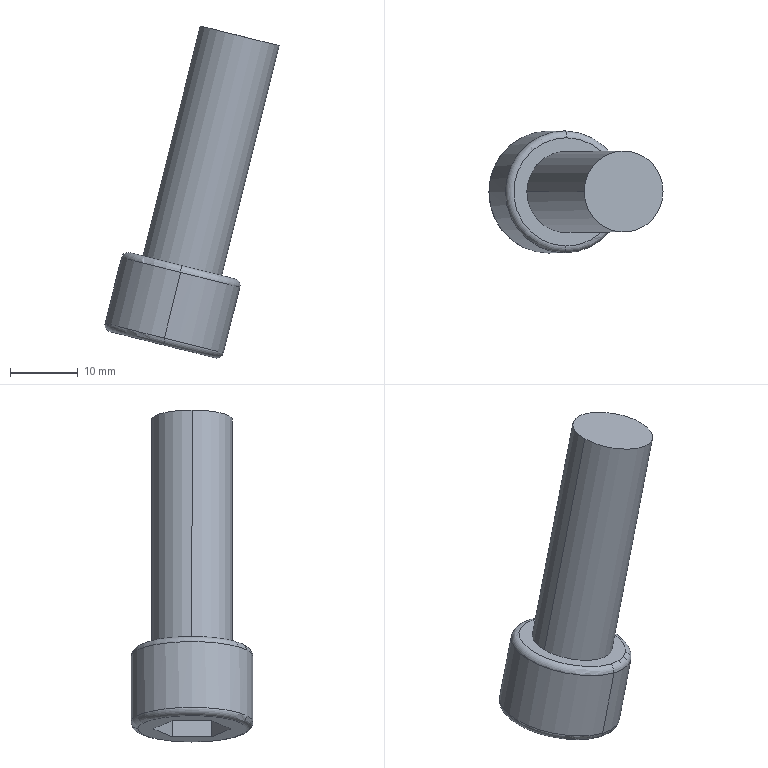Part | SolidWorks | features BaseBody 1 | 1 solid | 18 faces | box 25.711 x 18 x 49.02 mm | volume 6296 mm3 | plane 10 | torus 4 | cylinder 4 | commonest cylinder face diameters 12 x2 18 x2
STEP:
#1=CARTESIAN_POINT('',(-480.925,5.,189.664));
#2=VERTEX_POINT('',#1);
#3=CARTESIAN_POINT('',(-481.005,-13.,189.684));
#4=VERTEX_POINT('',#3);
#5=CARTESIAN_POINT('',(-480.925,-4.,189.664));
#6=DIRECTION('',(0.2419,0.,0.9703));
#7=DIRECTION('',(0.,-1.,0.));
#8=AXIS2_PLACEMENT_3D('',#5,#6,#7);
#9=CIRCLE('',#8,9.);
#10=EDGE_CURVE('',#2,#4,#9,.T.);
#11=ORIENTED_EDGE('',*,*,#10,.T.);
#12=CARTESIAN_POINT('',(-480.754,-12.,190.652));
#13=VERTEX_POINT('',#12);
#14=CARTESIAN_POINT('',(-480.996,-12.,189.681));
#15=DIRECTION('',(-0.9703,0.009133,0.2419));
#16=DIRECTION('',(0.2419,0.,0.9703));
#17=AXIS2_PLACEMENT_3D('',#14,#15,#16);
#18=CIRCLE('',#17,1.);
#19=EDGE_CURVE('',#4,#13,#18,.T.);
#20=ORIENTED_EDGE('',*,*,#19,.T.);
#21=CARTESIAN_POINT('',(-480.613,4.,190.616));
#22=VERTEX_POINT('',#21);
#23=CARTESIAN_POINT('',(-480.684,-4.,190.634));
#24=DIRECTION('',(0.2419,0.,0.9703));
#25=DIRECTION('',(0.,-1.,0.));
#26=AXIS2_PLACEMENT_3D('',#23,#24,#25);
#27=CIRCLE('',#26,8.);
#28=EDGE_CURVE('',#22,#13,#27,.T.);
#29=ORIENTED_EDGE('',*,*,#28,.F.);
#30=CARTESIAN_POINT('',(-480.846,5.,189.644));
#31=VERTEX_POINT('',#30);
#32=CARTESIAN_POINT('',(-480.855,4.,189.646));
#33=DIRECTION('',(0.9703,-0.009133,-0.2419));
#34=DIRECTION('',(-0.2419,0.,-0.9703));
#35=AXIS2_PLACEMENT_3D('',#32,#33,#34);
#36=CIRCLE('',#35,1.);
#37=EDGE_CURVE('',#31,#22,#36,.T.);
#38=ORIENTED_EDGE('',*,*,#37,.F.);
#39=CARTESIAN_POINT('',(-480.925,-4.,189.664));
#40=DIRECTION('',(0.2419,0.,0.9703));
#41=DIRECTION('',(0.,-1.,0.));
#42=AXIS2_PLACEMENT_3D('',#39,#40,#41);
#43=CIRCLE('',#42,9.);
#44=EDGE_CURVE('',#31,#2,#43,.T.);
#45=ORIENTED_EDGE('',*,*,#44,.T.);
#46=EDGE_LOOP('',(#11,#20,#29,#38,#45));
#47=FACE_OUTER_BOUND('',#46,.T.);
#48=CARTESIAN_POINT('',(-480.925,-4.,189.664));
#49=DIRECTION('',(0.2419,0.,0.9703));
#50=DIRECTION('',(0.008862,1.,-0.002209));
#51=AXIS2_PLACEMENT_3D('',#48,#49,#50);
#52=TOROIDAL_SURFACE('',#51,8.,1.);
#53=ADVANCED_FACE('',(#47),#52,.T.);
#54=CARTESIAN_POINT('',(-483.485,-11.999,178.965));
#55=VERTEX_POINT('',#54);
#56=CARTESIAN_POINT('',(-483.687,3.999,179.015));
#57=VERTEX_POINT('',#56);
#58=CARTESIAN_POINT('',(-483.586,-4.,178.99));
#59=DIRECTION('',(-0.2419,0.,-0.9703));
#60=DIRECTION('',(0.,-1.,0.));
#61=AXIS2_PLACEMENT_3D('',#58,#59,#60);
#62=CIRCLE('',#61,8.);
#63=EDGE_CURVE('',#55,#57,#62,.T.);
#64=ORIENTED_EDGE('',*,*,#63,.F.);
#65=CARTESIAN_POINT('',(-483.231,-12.999,179.932));
#66=VERTEX_POINT('',#65);
#67=CARTESIAN_POINT('',(-483.244,-11.999,179.936));
#68=DIRECTION('',(-0.9702,-0.01297,0.2419));
#69=DIRECTION('',(0.2419,0.,0.9703));
#70=AXIS2_PLACEMENT_3D('',#67,#68,#69);
#71=CIRCLE('',#70,1.);
#72=EDGE_CURVE('',#55,#66,#71,.T.);
#73=ORIENTED_EDGE('',*,*,#72,.T.);
#74=CARTESIAN_POINT('',(-483.344,-13.,179.961));
#75=VERTEX_POINT('',#74);
#76=CARTESIAN_POINT('',(-483.344,-4.,179.961));
#77=DIRECTION('',(-0.2419,0.,-0.9703));
#78=DIRECTION('',(0.,-1.,0.));
#79=AXIS2_PLACEMENT_3D('',#76,#77,#78);
#80=CIRCLE('',#79,9.);
#81=EDGE_CURVE('',#66,#75,#80,.T.);
#82=ORIENTED_EDGE('',*,*,#81,.T.);
#83=CARTESIAN_POINT('',(-483.458,4.999,179.989));
#84=VERTEX_POINT('',#83);
#85=CARTESIAN_POINT('',(-483.344,-4.,179.961));
#86=DIRECTION('',(-0.2419,0.,-0.9703));
#87=DIRECTION('',(0.,-1.,0.));
#88=AXIS2_PLACEMENT_3D('',#85,#86,#87);
#89=CIRCLE('',#88,9.);
#90=EDGE_CURVE('',#75,#84,#89,.T.);
#91=ORIENTED_EDGE('',*,*,#90,.T.);
#92=CARTESIAN_POINT('',(-483.445,3.999,179.986));
#93=DIRECTION('',(0.9702,0.01297,-0.2419));
#94=DIRECTION('',(-0.2419,0.,-0.9703));
#95=AXIS2_PLACEMENT_3D('',#92,#93,#94);
#96=CIRCLE('',#95,1.);
#97=EDGE_CURVE('',#57,#84,#96,.T.);
#98=ORIENTED_EDGE('',*,*,#97,.F.);
#99=EDGE_LOOP('',(#64,#73,#82,#91,#98));
#100=FACE_OUTER_BOUND('',#99,.T.);
#101=CARTESIAN_POINT('',(-483.344,-4.,179.961));
#102=DIRECTION('',(0.2419,0.,0.9703));
#103=DIRECTION('',(-0.01259,0.9999,0.003138));
#104=AXIS2_PLACEMENT_3D('',#101,#102,#103);
#105=TOROIDAL_SURFACE('',#104,8.,1.);
#106=ADVANCED_FACE('',(#100),#105,.T.);
#107=CARTESIAN_POINT('',(-483.344,5.,179.961));
#108=VERTEX_POINT('',#107);
#109=CARTESIAN_POINT('',(-483.344,-4.,179.961));
#110=DIRECTION('',(-0.2419,0.,-0.9703));
#111=DIRECTION('',(0.,-1.,0.));
#112=AXIS2_PLACEMENT_3D('',#109,#110,#111);
#113=CIRCLE('',#112,9.);
#114=EDGE_CURVE('',#108,#66,#113,.T.);
#115=ORIENTED_EDGE('',*,*,#114,.F.);
#116=CARTESIAN_POINT('',(-480.684,5.,190.634));
#117=DIRECTION('',(0.2419,0.,0.9703));
#118=VECTOR('',#117,1000.);
#119=LINE('',#116,#118);
#120=EDGE_CURVE('',#108,#2,#119,.T.);
#121=ORIENTED_EDGE('',*,*,#120,.T.);
#122=ORIENTED_EDGE('',*,*,#44,.F.);
#123=CARTESIAN_POINT('',(-480.925,-13.,189.664));
#124=VERTEX_POINT('',#123);
#125=CARTESIAN_POINT('',(-480.925,-4.,189.664));
#126=DIRECTION('',(0.2419,0.,0.9703));
#127=DIRECTION('',(0.,-1.,0.));
#128=AXIS2_PLACEMENT_3D('',#125,#126,#127);
#129=CIRCLE('',#128,9.);
#130=EDGE_CURVE('',#124,#31,#129,.T.);
#131=ORIENTED_EDGE('',*,*,#130,.F.);
#132=CARTESIAN_POINT('',(-480.684,-13.,190.634));
#133=DIRECTION('',(0.2419,0.,0.9703));
#134=VECTOR('',#133,1000.);
#135=LINE('',#132,#134);
#136=EDGE_CURVE('',#75,#124,#135,.T.);
#137=ORIENTED_EDGE('',*,*,#136,.F.);
#138=ORIENTED_EDGE('',*,*,#81,.F.);
#139=EDGE_LOOP('',(#115,#121,#122,#131,#137,#138));
#140=FACE_OUTER_BOUND('',#139,.T.);
#141=CARTESIAN_POINT('',(-480.684,-4.,190.634));
#142=DIRECTION('',(0.2419,0.,0.9703));
#143=DIRECTION('',(0.,-1.,0.));
#144=AXIS2_PLACEMENT_3D('',#141,#142,#143);
#145=CYLINDRICAL_SURFACE('',#144,9.);
#146=ADVANCED_FACE('',(#140),#145,.T.);
#147=CARTESIAN_POINT('',(-474.862,-4.,189.183));
#148=VERTEX_POINT('',#147);
#149=CARTESIAN_POINT('',(-486.505,-4.,192.085));
#150=VERTEX_POINT('',#149);
#151=CARTESIAN_POINT('',(-480.684,-4.,190.634));
#152=DIRECTION('',(0.2419,0.,0.9703));
#153=DIRECTION('',(0.9703,0.,-0.2419));
#154=AXIS2_PLACEMENT_3D('',#151,#152,#153);
#155=CIRCLE('',#154,6.);
#156=EDGE_CURVE('',#148,#150,#155,.T.);
#157=ORIENTED_EDGE('',*,*,#156,.T.);
#158=CARTESIAN_POINT('',(-478.039,-4.,226.046));
#159=VERTEX_POINT('',#158);
#160=CARTESIAN_POINT('',(-478.039,-4.,226.046));
#161=DIRECTION('',(0.2419,0.,0.9703));
#162=VECTOR('',#161,1000.);
#163=LINE('',#160,#162);
#164=EDGE_CURVE('',#150,#159,#163,.T.);
#165=ORIENTED_EDGE('',*,*,#164,.T.);
#166=CARTESIAN_POINT('',(-466.396,-4.,223.143));
#167=VERTEX_POINT('',#166);
#168=CARTESIAN_POINT('',(-472.218,-4.,224.595));
#169=DIRECTION('',(0.2419,0.,0.9703));
#170=DIRECTION('',(0.9703,0.,-0.2419));
#171=AXIS2_PLACEMENT_3D('',#168,#169,#170);
#172=CIRCLE('',#171,6.);
#173=EDGE_CURVE('',#167,#159,#172,.T.);
#174=ORIENTED_EDGE('',*,*,#173,.F.);
#175=CARTESIAN_POINT('',(-466.396,-4.,223.143));
#176=DIRECTION('',(0.2419,0.,0.9703));
#177=VECTOR('',#176,1000.);
#178=LINE('',#175,#177);
#179=EDGE_CURVE('',#148,#167,#178,.T.);
#180=ORIENTED_EDGE('',*,*,#179,.F.);
#181=EDGE_LOOP('',(#157,#165,#174,#180));
#182=FACE_OUTER_BOUND('',#181,.T.);
#183=CARTESIAN_POINT('',(-472.218,-4.,224.595));
#184=DIRECTION('',(0.2419,0.,0.9703));
#185=DIRECTION('',(0.9703,0.,-0.2419));
#186=AXIS2_PLACEMENT_3D('',#183,#184,#185);
#187=CYLINDRICAL_SURFACE('',#186,6.);
#188=ADVANCED_FACE('',(#182),#187,.T.);
#189=ORIENTED_EDGE('',*,*,#156,.F.);
#190=CARTESIAN_POINT('',(-480.684,-4.,190.634));
#191=DIRECTION('',(0.2419,0.,0.9703));
#192=DIRECTION('',(0.9703,0.,-0.2419));
#193=AXIS2_PLACEMENT_3D('',#190,#191,#192);
#194=CIRCLE('',#193,6.);
#195=EDGE_CURVE('',#150,#148,#194,.T.);
#196=ORIENTED_EDGE('',*,*,#195,.F.);
#197=EDGE_LOOP('',(#189,#196));
#198=FACE_BOUND('',#197,.T.);
#199=ORIENTED_EDGE('',*,*,#28,.T.);
#200=CARTESIAN_POINT('',(-480.684,-4.,190.634));
#201=DIRECTION('',(0.2419,0.,0.9703));
#202=DIRECTION('',(0.,-1.,0.));
#203=AXIS2_PLACEMENT_3D('',#200,#201,#202);
#204=CIRCLE('',#203,8.);
#205=EDGE_CURVE('',#13,#22,#204,.T.);
#206=ORIENTED_EDGE('',*,*,#205,.T.);
#207=EDGE_LOOP('',(#199,#206));
#208=FACE_OUTER_BOUND('',#207,.T.);
#209=CARTESIAN_POINT('',(-480.684,-4.,190.634));
#210=DIRECTION('',(0.2419,0.,0.9703));
#211=DIRECTION('',(0.,-1.,0.));
#212=AXIS2_PLACEMENT_3D('',#209,#210,#211);
#213=PLANE('',#212);
#214=ADVANCED_FACE('',(#198,#208),#213,.T.);
#215=ORIENTED_EDGE('',*,*,#164,.F.);
#216=ORIENTED_EDGE('',*,*,#195,.T.);
#217=ORIENTED_EDGE('',*,*,#179,.T.);
#218=CARTESIAN_POINT('',(-472.218,-4.,224.595));
#219=DIRECTION('',(0.2419,0.,0.9703));
#220=DIRECTION('',(0.9703,0.,-0.2419));
#221=AXIS2_PLACEMENT_3D('',#218,#219,#220);
#222=CIRCLE('',#221,6.);
#223=EDGE_CURVE('',#159,#167,#222,.T.);
#224=ORIENTED_EDGE('',*,*,#223,.F.);
#225=EDGE_LOOP('',(#215,#216,#217,#224));
#226=FACE_OUTER_BOUND('',#225,.T.);
#227=CARTESIAN_POINT('',(-472.218,-4.,224.595));
#228=DIRECTION('',(0.2419,0.,0.9703));
#229=DIRECTION('',(0.9703,0.,-0.2419));
#230=AXIS2_PLACEMENT_3D('',#227,#228,#229);
#231=CYLINDRICAL_SURFACE('',#230,6.);
#232=ADVANCED_FACE('',(#226),#231,.T.);
#233=ORIENTED_EDGE('',*,*,#173,.T.);
#234=ORIENTED_EDGE('',*,*,#223,.T.);
#235=EDGE_LOOP('',(#233,#234));
#236=FACE_OUTER_BOUND('',#235,.T.);
#237=CARTESIAN_POINT('',(-472.218,-4.,224.595));
#238=DIRECTION('',(0.2419,0.,0.9703));
#239=DIRECTION('',(0.,-1.,0.));
#240=AXIS2_PLACEMENT_3D('',#237,#238,#239);
#241=PLANE('',#240);
#242=ADVANCED_FACE('',(#236),#241,.T.);
#243=CARTESIAN_POINT('',(-483.586,1.774,178.99));
#244=VERTEX_POINT('',#243);
#245=CARTESIAN_POINT('',(-478.735,-1.113,177.781));
#246=VERTEX_POINT('',#245);
#247=CARTESIAN_POINT('',(-483.586,1.774,178.99));
#248=DIRECTION('',(0.8403,-0.5,-0.2095));
#249=VECTOR('',#248,1000.);
#250=LINE('',#247,#249);
#251=EDGE_CURVE('',#244,#246,#250,.T.);
#252=ORIENTED_EDGE('',*,*,#251,.F.);
#253=CARTESIAN_POINT('',(-488.438,-1.113,180.2));
#254=VERTEX_POINT('',#253);
#255=CARTESIAN_POINT('',(-488.438,-1.113,180.2));
#256=DIRECTION('',(0.8403,0.5,-0.2095));
#257=VECTOR('',#256,1000.);
#258=LINE('',#255,#257);
#259=EDGE_CURVE('',#254,#244,#258,.T.);
#260=ORIENTED_EDGE('',*,*,#259,.F.);
#261=CARTESIAN_POINT('',(-488.438,-6.887,180.2));
#262=VERTEX_POINT('',#261);
#263=CARTESIAN_POINT('',(-488.438,-6.887,180.2));
#264=DIRECTION('',(0.,1.,0.));
#265=VECTOR('',#264,1000.);
#266=LINE('',#263,#265);
#267=EDGE_CURVE('',#262,#254,#266,.T.);
#268=ORIENTED_EDGE('',*,*,#267,.F.);
#269=CARTESIAN_POINT('',(-483.586,-9.774,178.99));
#270=VERTEX_POINT('',#269);
#271=CARTESIAN_POINT('',(-483.586,-9.774,178.99));
#272=DIRECTION('',(-0.8403,0.5,0.2095));
#273=VECTOR('',#272,1000.);
#274=LINE('',#271,#273);
#275=EDGE_CURVE('',#270,#262,#274,.T.);
#276=ORIENTED_EDGE('',*,*,#275,.F.);
#277=CARTESIAN_POINT('',(-478.735,-6.887,177.781));
#278=VERTEX_POINT('',#277);
#279=CARTESIAN_POINT('',(-478.735,-6.887,177.781));
#280=DIRECTION('',(-0.8403,-0.5,0.2095));
#281=VECTOR('',#280,1000.);
#282=LINE('',#279,#281);
#283=EDGE_CURVE('',#278,#270,#282,.T.);
#284=ORIENTED_EDGE('',*,*,#283,.F.);
#285=CARTESIAN_POINT('',(-478.735,-1.113,177.781));
#286=DIRECTION('',(0.,-1.,0.));
#287=VECTOR('',#286,1000.);
#288=LINE('',#285,#287);
#289=EDGE_CURVE('',#246,#278,#288,.T.);
#290=ORIENTED_EDGE('',*,*,#289,.F.);
#291=EDGE_LOOP('',(#252,#260,#268,#276,#284,#290));
#292=FACE_BOUND('',#291,.T.);
#293=CARTESIAN_POINT('',(-483.586,-4.,178.99));
#294=DIRECTION('',(-0.2419,0.,-0.9703));
#295=DIRECTION('',(0.,-1.,0.));
#296=AXIS2_PLACEMENT_3D('',#293,#294,#295);
#297=CIRCLE('',#296,8.);
#298=EDGE_CURVE('',#57,#55,#297,.T.);
#299=ORIENTED_EDGE('',*,*,#298,.T.);
#300=ORIENTED_EDGE('',*,*,#63,.T.);
#301=EDGE_LOOP('',(#299,#300));
#302=FACE_OUTER_BOUND('',#301,.T.);
#303=CARTESIAN_POINT('',(-483.586,-4.,178.99));
#304=DIRECTION('',(0.2419,0.,0.9703));
#305=DIRECTION('',(0.,-1.,0.));
#306=AXIS2_PLACEMENT_3D('',#303,#304,#305);
#307=PLANE('',#306);
#308=ADVANCED_FACE('',(#292,#302),#307,.F.);
#309=CARTESIAN_POINT('',(-476.8,-6.887,185.543));
#310=VERTEX_POINT('',#309);
#311=CARTESIAN_POINT('',(-478.735,-6.887,177.781));
#312=DIRECTION('',(0.2419,0.,0.9703));
#313=VECTOR('',#312,1000.);
#314=LINE('',#311,#313);
#315=EDGE_CURVE('',#278,#310,#314,.T.);
#316=ORIENTED_EDGE('',*,*,#315,.T.);
#317=CARTESIAN_POINT('',(-476.8,-1.113,185.543));
#318=VERTEX_POINT('',#317);
#319=CARTESIAN_POINT('',(-476.8,-1.113,185.543));
#320=DIRECTION('',(0.,-1.,0.));
#321=VECTOR('',#320,1000.);
#322=LINE('',#319,#321);
#323=EDGE_CURVE('',#318,#310,#322,.T.);
#324=ORIENTED_EDGE('',*,*,#323,.F.);
#325=CARTESIAN_POINT('',(-478.735,-1.113,177.781));
#326=DIRECTION('',(0.2419,0.,0.9703));
#327=VECTOR('',#326,1000.);
#328=LINE('',#325,#327);
#329=EDGE_CURVE('',#246,#318,#328,.T.);
#330=ORIENTED_EDGE('',*,*,#329,.F.);
#331=ORIENTED_EDGE('',*,*,#289,.T.);
#332=EDGE_LOOP('',(#316,#324,#330,#331));
#333=FACE_OUTER_BOUND('',#332,.T.);
#334=CARTESIAN_POINT('',(-478.735,-1.113,177.781));
#335=DIRECTION('',(0.9703,0.,-0.2419));
#336=DIRECTION('',(0.,-1.,0.));
#337=AXIS2_PLACEMENT_3D('',#334,#335,#336);
#338=PLANE('',#337);
#339=ADVANCED_FACE('',(#333),#338,.F.);
#340=ORIENTED_EDGE('',*,*,#329,.T.);
#341=CARTESIAN_POINT('',(-481.651,1.774,186.753));
#342=VERTEX_POINT('',#341);
#343=CARTESIAN_POINT('',(-481.651,1.774,186.753));
#344=DIRECTION('',(0.8403,-0.5,-0.2095));
#345=VECTOR('',#344,1000.);
#346=LINE('',#343,#345);
#347=EDGE_CURVE('',#342,#318,#346,.T.);
#348=ORIENTED_EDGE('',*,*,#347,.F.);
#349=CARTESIAN_POINT('',(-483.586,1.774,178.99));
#350=DIRECTION('',(0.2419,0.,0.9703));
#351=VECTOR('',#350,1000.);
#352=LINE('',#349,#351);
#353=EDGE_CURVE('',#244,#342,#352,.T.);
#354=ORIENTED_EDGE('',*,*,#353,.F.);
#355=ORIENTED_EDGE('',*,*,#251,.T.);
#356=EDGE_LOOP('',(#340,#348,#354,#355));
#357=FACE_OUTER_BOUND('',#356,.T.);
#358=CARTESIAN_POINT('',(-483.586,1.774,178.99));
#359=DIRECTION('',(0.4852,0.866,-0.1209));
#360=DIRECTION('',(-0.2419,0.,-0.9703));
#361=AXIS2_PLACEMENT_3D('',#358,#359,#360);
#362=PLANE('',#361);
#363=ADVANCED_FACE('',(#357),#362,.F.);
#364=ORIENTED_EDGE('',*,*,#353,.T.);
#365=CARTESIAN_POINT('',(-486.503,-1.113,187.962));
#366=VERTEX_POINT('',#365);
#367=CARTESIAN_POINT('',(-486.503,-1.113,187.962));
#368=DIRECTION('',(0.8403,0.5,-0.2095));
#369=VECTOR('',#368,1000.);
#370=LINE('',#367,#369);
#371=EDGE_CURVE('',#366,#342,#370,.T.);
#372=ORIENTED_EDGE('',*,*,#371,.F.);
#373=CARTESIAN_POINT('',(-488.438,-1.113,180.2));
#374=DIRECTION('',(0.2419,0.,0.9703));
#375=VECTOR('',#374,1000.);
#376=LINE('',#373,#375);
#377=EDGE_CURVE('',#254,#366,#376,.T.);
#378=ORIENTED_EDGE('',*,*,#377,.F.);
#379=ORIENTED_EDGE('',*,*,#259,.T.);
#380=EDGE_LOOP('',(#364,#372,#378,#379));
#381=FACE_OUTER_BOUND('',#380,.T.);
#382=CARTESIAN_POINT('',(-488.438,-1.113,180.2));
#383=DIRECTION('',(-0.4852,0.866,0.1209));
#384=DIRECTION('',(0.2419,0.,0.9703));
#385=AXIS2_PLACEMENT_3D('',#382,#383,#384);
#386=PLANE('',#385);
#387=ADVANCED_FACE('',(#381),#386,.F.);
#388=ORIENTED_EDGE('',*,*,#377,.T.);
#389=CARTESIAN_POINT('',(-486.503,-6.887,187.962));
#390=VERTEX_POINT('',#389);
#391=CARTESIAN_POINT('',(-486.503,-6.887,187.962));
#392=DIRECTION('',(0.,1.,0.));
#393=VECTOR('',#392,1000.);
#394=LINE('',#391,#393);
#395=EDGE_CURVE('',#390,#366,#394,.T.);
#396=ORIENTED_EDGE('',*,*,#395,.F.);
#397=CARTESIAN_POINT('',(-488.438,-6.887,180.2));
#398=DIRECTION('',(0.2419,0.,0.9703));
#399=VECTOR('',#398,1000.);
#400=LINE('',#397,#399);
#401=EDGE_CURVE('',#262,#390,#400,.T.);
#402=ORIENTED_EDGE('',*,*,#401,.F.);
#403=ORIENTED_EDGE('',*,*,#267,.T.);
#404=EDGE_LOOP('',(#388,#396,#402,#403));
#405=FACE_OUTER_BOUND('',#404,.T.);
#406=CARTESIAN_POINT('',(-488.438,-6.887,180.2));
#407=DIRECTION('',(-0.9703,0.,0.2419));
#408=DIRECTION('',(0.,1.,0.));
#409=AXIS2_PLACEMENT_3D('',#406,#407,#408);
#410=PLANE('',#409);
#411=ADVANCED_FACE('',(#405),#410,.F.);
#412=ORIENTED_EDGE('',*,*,#401,.T.);
#413=CARTESIAN_POINT('',(-481.651,-9.774,186.753));
#414=VERTEX_POINT('',#413);
#415=CARTESIAN_POINT('',(-481.651,-9.774,186.753));
#416=DIRECTION('',(-0.8403,0.5,0.2095));
#417=VECTOR('',#416,1000.);
#418=LINE('',#415,#417);
#419=EDGE_CURVE('',#414,#390,#418,.T.);
#420=ORIENTED_EDGE('',*,*,#419,.F.);
#421=CARTESIAN_POINT('',(-483.586,-9.774,178.99));
#422=DIRECTION('',(0.2419,0.,0.9703));
#423=VECTOR('',#422,1000.);
#424=LINE('',#421,#423);
#425=EDGE_CURVE('',#270,#414,#424,.T.);
#426=ORIENTED_EDGE('',*,*,#425,.F.);
#427=ORIENTED_EDGE('',*,*,#275,.T.);
#428=EDGE_LOOP('',(#412,#420,#426,#427));
#429=FACE_OUTER_BOUND('',#428,.T.);
#430=CARTESIAN_POINT('',(-483.586,-9.774,178.99));
#431=DIRECTION('',(-0.4852,-0.866,0.1209));
#432=DIRECTION('',(-0.8724,0.4887,0.));
#433=AXIS2_PLACEMENT_3D('',#430,#431,#432);
#434=PLANE('',#433);
#435=ADVANCED_FACE('',(#429),#434,.F.);
#436=ORIENTED_EDGE('',*,*,#425,.T.);
#437=CARTESIAN_POINT('',(-476.8,-6.887,185.543));
#438=DIRECTION('',(-0.8403,-0.5,0.2095));
#439=VECTOR('',#438,1000.);
#440=LINE('',#437,#439);
#441=EDGE_CURVE('',#310,#414,#440,.T.);
#442=ORIENTED_EDGE('',*,*,#441,.F.);
#443=ORIENTED_EDGE('',*,*,#315,.F.);
#444=ORIENTED_EDGE('',*,*,#283,.T.);
#445=EDGE_LOOP('',(#436,#442,#443,#444));
#446=FACE_OUTER_BOUND('',#445,.T.);
#447=CARTESIAN_POINT('',(-478.735,-6.887,177.781));
#448=DIRECTION('',(0.4852,-0.866,-0.1209));
#449=DIRECTION('',(0.,0.1383,-0.9904));
#450=AXIS2_PLACEMENT_3D('',#447,#448,#449);
#451=PLANE('',#450);
#452=ADVANCED_FACE('',(#446),#451,.F.);
#453=ORIENTED_EDGE('',*,*,#441,.T.);
#454=ORIENTED_EDGE('',*,*,#419,.T.);
#455=ORIENTED_EDGE('',*,*,#395,.T.);
#456=ORIENTED_EDGE('',*,*,#371,.T.);
#457=ORIENTED_EDGE('',*,*,#347,.T.);
#458=ORIENTED_EDGE('',*,*,#323,.T.);
#459=EDGE_LOOP('',(#453,#454,#455,#456,#457,#458));
#460=FACE_OUTER_BOUND('',#459,.T.);
#461=CARTESIAN_POINT('',(-481.651,-4.,186.753));
#462=DIRECTION('',(-0.2419,0.,-0.9703));
#463=DIRECTION('',(-0.9703,0.,0.2419));
#464=AXIS2_PLACEMENT_3D('',#461,#462,#463);
#465=PLANE('',#464);
#466=ADVANCED_FACE('',(#460),#465,.T.);
#467=ORIENTED_EDGE('',*,*,#120,.F.);
#468=CARTESIAN_POINT('',(-483.344,-4.,179.961));
#469=DIRECTION('',(-0.2419,0.,-0.9703));
#470=DIRECTION('',(0.,-1.,0.));
#471=AXIS2_PLACEMENT_3D('',#468,#469,#470);
#472=CIRCLE('',#471,9.);
#473=EDGE_CURVE('',#84,#108,#472,.T.);
#474=ORIENTED_EDGE('',*,*,#473,.F.);
#475=ORIENTED_EDGE('',*,*,#90,.F.);
#476=ORIENTED_EDGE('',*,*,#136,.T.);
#477=CARTESIAN_POINT('',(-480.925,-4.,189.664));
#478=DIRECTION('',(0.2419,0.,0.9703));
#479=DIRECTION('',(0.,-1.,0.));
#480=AXIS2_PLACEMENT_3D('',#477,#478,#479);
#481=CIRCLE('',#480,9.);
#482=EDGE_CURVE('',#4,#124,#481,.T.);
#483=ORIENTED_EDGE('',*,*,#482,.F.);
#484=ORIENTED_EDGE('',*,*,#10,.F.);
#485=EDGE_LOOP('',(#467,#474,#475,#476,#483,#484));
#486=FACE_OUTER_BOUND('',#485,.T.);
#487=CARTESIAN_POINT('',(-480.684,-4.,190.634));
#488=DIRECTION('',(0.2419,0.,0.9703));
#489=DIRECTION('',(0.,-1.,0.));
#490=AXIS2_PLACEMENT_3D('',#487,#488,#489);
#491=CYLINDRICAL_SURFACE('',#490,9.);
#492=ADVANCED_FACE('',(#486),#491,.T.);
#493=ORIENTED_EDGE('',*,*,#72,.F.);
#494=ORIENTED_EDGE('',*,*,#298,.F.);
#495=ORIENTED_EDGE('',*,*,#97,.T.);
#496=ORIENTED_EDGE('',*,*,#473,.T.);
#497=ORIENTED_EDGE('',*,*,#114,.T.);
#498=EDGE_LOOP('',(#493,#494,#495,#496,#497));
#499=FACE_OUTER_BOUND('',#498,.T.);
#500=CARTESIAN_POINT('',(-483.344,-4.,179.961));
#501=DIRECTION('',(0.2419,0.,0.9703));
#502=DIRECTION('',(-0.01259,0.9999,0.003138));
#503=AXIS2_PLACEMENT_3D('',#500,#501,#502);
#504=TOROIDAL_SURFACE('',#503,8.,1.);
#505=ADVANCED_FACE('',(#499),#504,.T.);
#506=ORIENTED_EDGE('',*,*,#19,.F.);
#507=ORIENTED_EDGE('',*,*,#482,.T.);
#508=ORIENTED_EDGE('',*,*,#130,.T.);
#509=ORIENTED_EDGE('',*,*,#37,.T.);
#510=ORIENTED_EDGE('',*,*,#205,.F.);
#511=EDGE_LOOP('',(#506,#507,#508,#509,#510));
#512=FACE_OUTER_BOUND('',#511,.T.);
#513=CARTESIAN_POINT('',(-480.925,-4.,189.664));
#514=DIRECTION('',(0.2419,0.,0.9703));
#515=DIRECTION('',(0.008862,1.,-0.002209));
#516=AXIS2_PLACEMENT_3D('',#513,#514,#515);
#517=TOROIDAL_SURFACE('',#516,8.,1.);
#518=ADVANCED_FACE('',(#512),#517,.T.);
#519=CLOSED_SHELL('',(#53,#106,#146,#188,#214,#232,#242,#308,#339,#363,#387,#411,#435,#452,#466,#492,#505,#518));
#520=MANIFOLD_SOLID_BREP('',#519);
#521=CARTESIAN_POINT('',(0.,0.,0.));
#522=DIRECTION('',(0.,0.,1.));
#523=DIRECTION('',(1.,0.,0.));
#524=AXIS2_PLACEMENT_3D('',#521,#522,#523);
#525=(LENGTH_UNIT()NAMED_UNIT(*)SI_UNIT(.MILLI.,.METRE.));
#526=UNCERTAINTY_MEASURE_WITH_UNIT(LENGTH_MEASURE(0.00001),#525,'','');
#527=(NAMED_UNIT(*)PLANE_ANGLE_UNIT()SI_UNIT($,.RADIAN.));
#528=(NAMED_UNIT(*)SI_UNIT($,.STERADIAN.)SOLID_ANGLE_UNIT());
#529=(GEOMETRIC_REPRESENTATION_CONTEXT(3)GLOBAL_UNCERTAINTY_ASSIGNED_CONTEXT((#526))GLOBAL_UNIT_ASSIGNED_CONTEXT((#525,#527,#528))REPRESENTATION_CONTEXT('',''));
#530=ADVANCED_BREP_SHAPE_REPRESENTATION('',(#520,#524),#529);